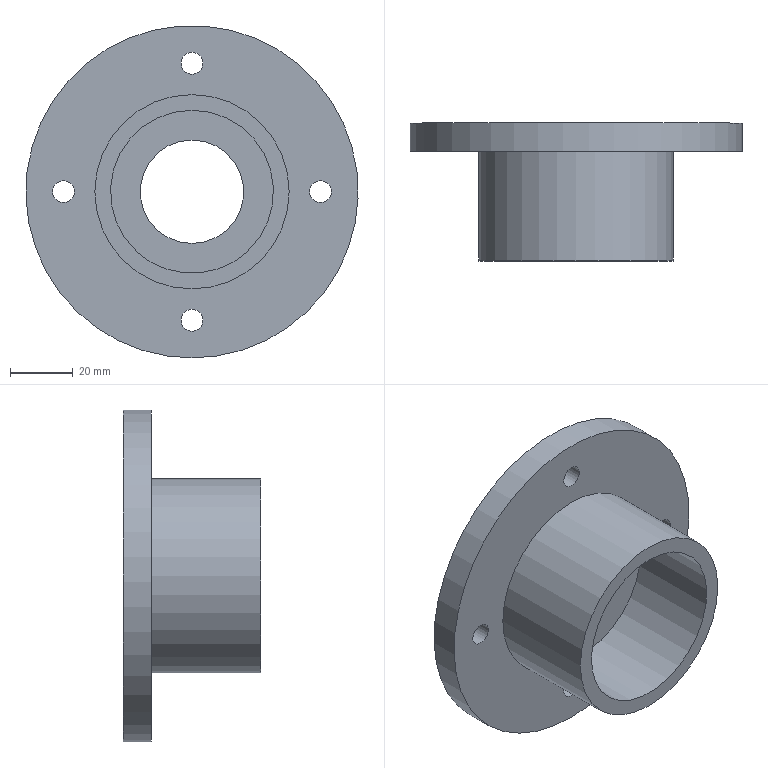Part | NX | features DATUM_CSYS 8, HOLE PACKAGE 7, SIMPLE HOLE 7, SKETCH 7, EXTRACT_DATUM_AXIS 4, EXTRACT_FACE 4, Instance Feature 3, EXTRUDE 2, OFFSET_REGION 1, Pattern Feature 1, SWP104 1 | 1 solid | 18 faces | box 106 x 44 x 106 mm | volume 98017 mm3 | cylinder 11 | plane 5 | cone 2 | commonest cylinder face diameters 7 x4 33 x2 48 x1 52 x1 58 x1 62 x1
STEP:
#1=CARTESIAN_POINT('',(0.,-14.,16.5));
#2=VERTEX_POINT('',#1);
#3=CARTESIAN_POINT('',(0.,-14.,0.));
#4=DIRECTION('',(0.,1.,0.));
#5=DIRECTION('',(0.,0.,1.));
#6=AXIS2_PLACEMENT_3D('',#3,#4,#5);
#7=CIRCLE('',#6,16.5);
#8=EDGE_CURVE('',#2,#2,#7,.T.);
#9=ORIENTED_EDGE('',*,*,#8,.F.);
#10=EDGE_LOOP('',(#9));
#11=FACE_BOUND('',#10,.T.);
#12=CARTESIAN_POINT('',(0.,-9.169,16.5));
#13=VERTEX_POINT('',#12);
#14=CARTESIAN_POINT('',(0.,-9.169,0.));
#15=DIRECTION('',(0.,1.,0.));
#16=DIRECTION('',(0.,0.,1.));
#17=AXIS2_PLACEMENT_3D('',#14,#15,#16);
#18=CIRCLE('',#17,16.5);
#19=EDGE_CURVE('',#13,#13,#18,.F.);
#20=ORIENTED_EDGE('',*,*,#19,.F.);
#21=EDGE_LOOP('',(#20));
#22=FACE_BOUND('',#21,.T.);
#23=CARTESIAN_POINT('',(0.,-44.,0.));
#24=DIRECTION('',(0.,1.,0.));
#25=DIRECTION('',(0.,0.,1.));
#26=AXIS2_PLACEMENT_3D('',#23,#24,#25);
#27=CYLINDRICAL_SURFACE('',#26,16.5);
#28=ADVANCED_FACE('',(#11,#22),#27,.F.);
#29=CARTESIAN_POINT('',(0.,-3.,-16.5));
#30=VERTEX_POINT('',#29);
#31=CARTESIAN_POINT('',(0.,-3.,0.));
#32=DIRECTION('',(0.,-1.,0.));
#33=DIRECTION('',(0.,0.,-1.));
#34=AXIS2_PLACEMENT_3D('',#31,#32,#33);
#35=CIRCLE('',#34,16.5);
#36=EDGE_CURVE('',#30,#30,#35,.F.);
#37=ORIENTED_EDGE('',*,*,#36,.T.);
#38=EDGE_LOOP('',(#37));
#39=FACE_BOUND('',#38,.T.);
#40=CARTESIAN_POINT('',(0.,-3.327,-16.5));
#41=VERTEX_POINT('',#40);
#42=CARTESIAN_POINT('',(0.,-3.327,0.));
#43=DIRECTION('',(0.,-1.,0.));
#44=DIRECTION('',(0.,0.,-1.));
#45=AXIS2_PLACEMENT_3D('',#42,#43,#44);
#46=CIRCLE('',#45,16.5);
#47=EDGE_CURVE('',#41,#41,#46,.F.);
#48=ORIENTED_EDGE('',*,*,#47,.F.);
#49=EDGE_LOOP('',(#48));
#50=FACE_BOUND('',#49,.T.);
#51=CARTESIAN_POINT('',(0.,-44.,0.));
#52=DIRECTION('',(0.,1.,0.));
#53=DIRECTION('',(0.,0.,1.));
#54=AXIS2_PLACEMENT_3D('',#51,#52,#53);
#55=CYLINDRICAL_SURFACE('',#54,16.5);
#56=ADVANCED_FACE('',(#39,#50),#55,.F.);
#57=CARTESIAN_POINT('',(0.,-9.,-53.));
#58=VERTEX_POINT('',#57);
#59=CARTESIAN_POINT('',(0.,-9.,0.));
#60=DIRECTION('',(0.,-1.,0.));
#61=DIRECTION('',(0.,0.,-1.));
#62=AXIS2_PLACEMENT_3D('',#59,#60,#61);
#63=CIRCLE('',#62,53.);
#64=EDGE_CURVE('',#58,#58,#63,.T.);
#65=ORIENTED_EDGE('',*,*,#64,.F.);
#66=EDGE_LOOP('',(#65));
#67=FACE_BOUND('',#66,.T.);
#68=CARTESIAN_POINT('',(0.,0.,-53.));
#69=VERTEX_POINT('',#68);
#70=CARTESIAN_POINT('',(0.,0.,0.));
#71=DIRECTION('',(0.,-1.,0.));
#72=DIRECTION('',(0.,0.,-1.));
#73=AXIS2_PLACEMENT_3D('',#70,#71,#72);
#74=CIRCLE('',#73,53.);
#75=EDGE_CURVE('',#69,#69,#74,.T.);
#76=ORIENTED_EDGE('',*,*,#75,.T.);
#77=EDGE_LOOP('',(#76));
#78=FACE_BOUND('',#77,.T.);
#79=CARTESIAN_POINT('',(0.,-9.,0.));
#80=DIRECTION('',(0.,1.,0.));
#81=DIRECTION('',(0.,0.,1.));
#82=AXIS2_PLACEMENT_3D('',#79,#80,#81);
#83=CYLINDRICAL_SURFACE('',#82,53.);
#84=ADVANCED_FACE('',(#67,#78),#83,.T.);
#85=CARTESIAN_POINT('',(0.,-9.,-44.5));
#86=VERTEX_POINT('',#85);
#87=CARTESIAN_POINT('',(0.,-9.,-41.));
#88=DIRECTION('',(0.,-1.,0.));
#89=DIRECTION('',(0.,0.,-1.));
#90=AXIS2_PLACEMENT_3D('',#87,#88,#89);
#91=CIRCLE('',#90,3.5);
#92=EDGE_CURVE('',#86,#86,#91,.T.);
#93=ORIENTED_EDGE('',*,*,#92,.F.);
#94=EDGE_LOOP('',(#93));
#95=FACE_BOUND('',#94,.T.);
#96=CARTESIAN_POINT('',(41.,-9.,-3.5));
#97=VERTEX_POINT('',#96);
#98=CARTESIAN_POINT('',(41.,-9.,0.));
#99=DIRECTION('',(0.,-1.,0.));
#100=DIRECTION('',(0.,0.,-1.));
#101=AXIS2_PLACEMENT_3D('',#98,#99,#100);
#102=CIRCLE('',#101,3.5);
#103=EDGE_CURVE('',#97,#97,#102,.T.);
#104=ORIENTED_EDGE('',*,*,#103,.F.);
#105=EDGE_LOOP('',(#104));
#106=FACE_BOUND('',#105,.T.);
#107=CARTESIAN_POINT('',(0.,-9.,37.5));
#108=VERTEX_POINT('',#107);
#109=CARTESIAN_POINT('',(0.,-9.,41.));
#110=DIRECTION('',(0.,-1.,0.));
#111=DIRECTION('',(0.,0.,-1.));
#112=AXIS2_PLACEMENT_3D('',#109,#110,#111);
#113=CIRCLE('',#112,3.5);
#114=EDGE_CURVE('',#108,#108,#113,.T.);
#115=ORIENTED_EDGE('',*,*,#114,.F.);
#116=EDGE_LOOP('',(#115));
#117=FACE_BOUND('',#116,.T.);
#118=CARTESIAN_POINT('',(-41.,-9.,-3.5));
#119=VERTEX_POINT('',#118);
#120=CARTESIAN_POINT('',(-41.,-9.,0.));
#121=DIRECTION('',(0.,-1.,0.));
#122=DIRECTION('',(0.,0.,-1.));
#123=AXIS2_PLACEMENT_3D('',#120,#121,#122);
#124=CIRCLE('',#123,3.5);
#125=EDGE_CURVE('',#119,#119,#124,.T.);
#126=ORIENTED_EDGE('',*,*,#125,.F.);
#127=EDGE_LOOP('',(#126));
#128=FACE_BOUND('',#127,.T.);
#129=CARTESIAN_POINT('',(31.,-9.,0.));
#130=VERTEX_POINT('',#129);
#131=CARTESIAN_POINT('',(0.,-9.,0.));
#132=DIRECTION('',(0.,-1.,0.));
#133=DIRECTION('',(1.,0.,0.));
#134=AXIS2_PLACEMENT_3D('',#131,#132,#133);
#135=CIRCLE('',#134,31.);
#136=EDGE_CURVE('',#130,#130,#135,.T.);
#137=ORIENTED_EDGE('',*,*,#136,.F.);
#138=EDGE_LOOP('',(#137));
#139=FACE_BOUND('',#138,.T.);
#140=ORIENTED_EDGE('',*,*,#64,.T.);
#141=EDGE_LOOP('',(#140));
#142=FACE_BOUND('',#141,.T.);
#143=CARTESIAN_POINT('',(0.,-9.,0.));
#144=DIRECTION('',(0.,-1.,0.));
#145=DIRECTION('',(0.,0.,-1.));
#146=AXIS2_PLACEMENT_3D('',#143,#144,#145);
#147=PLANE('',#146);
#148=ADVANCED_FACE('',(#95,#106,#117,#128,#139,#142),#147,.T.);
#149=CARTESIAN_POINT('',(0.,0.,-44.5));
#150=VERTEX_POINT('',#149);
#151=CARTESIAN_POINT('',(0.,0.,-41.));
#152=DIRECTION('',(0.,-1.,0.));
#153=DIRECTION('',(0.,0.,-1.));
#154=AXIS2_PLACEMENT_3D('',#151,#152,#153);
#155=CIRCLE('',#154,3.5);
#156=EDGE_CURVE('',#150,#150,#155,.T.);
#157=ORIENTED_EDGE('',*,*,#156,.T.);
#158=EDGE_LOOP('',(#157));
#159=FACE_BOUND('',#158,.T.);
#160=CARTESIAN_POINT('',(41.,0.,-3.5));
#161=VERTEX_POINT('',#160);
#162=CARTESIAN_POINT('',(41.,0.,0.));
#163=DIRECTION('',(0.,-1.,0.));
#164=DIRECTION('',(0.,0.,-1.));
#165=AXIS2_PLACEMENT_3D('',#162,#163,#164);
#166=CIRCLE('',#165,3.5);
#167=EDGE_CURVE('',#161,#161,#166,.T.);
#168=ORIENTED_EDGE('',*,*,#167,.T.);
#169=EDGE_LOOP('',(#168));
#170=FACE_BOUND('',#169,.T.);
#171=CARTESIAN_POINT('',(0.,0.,37.5));
#172=VERTEX_POINT('',#171);
#173=CARTESIAN_POINT('',(0.,0.,41.));
#174=DIRECTION('',(0.,-1.,0.));
#175=DIRECTION('',(0.,0.,-1.));
#176=AXIS2_PLACEMENT_3D('',#173,#174,#175);
#177=CIRCLE('',#176,3.5);
#178=EDGE_CURVE('',#172,#172,#177,.T.);
#179=ORIENTED_EDGE('',*,*,#178,.T.);
#180=EDGE_LOOP('',(#179));
#181=FACE_BOUND('',#180,.T.);
#182=CARTESIAN_POINT('',(-41.,0.,-3.5));
#183=VERTEX_POINT('',#182);
#184=CARTESIAN_POINT('',(-41.,0.,0.));
#185=DIRECTION('',(0.,-1.,0.));
#186=DIRECTION('',(0.,0.,-1.));
#187=AXIS2_PLACEMENT_3D('',#184,#185,#186);
#188=CIRCLE('',#187,3.5);
#189=EDGE_CURVE('',#183,#183,#188,.T.);
#190=ORIENTED_EDGE('',*,*,#189,.T.);
#191=EDGE_LOOP('',(#190));
#192=FACE_BOUND('',#191,.T.);
#193=CARTESIAN_POINT('',(0.,0.,-29.));
#194=VERTEX_POINT('',#193);
#195=CARTESIAN_POINT('',(0.,0.,0.));
#196=DIRECTION('',(0.,-1.,0.));
#197=DIRECTION('',(0.,0.,-1.));
#198=AXIS2_PLACEMENT_3D('',#195,#196,#197);
#199=CIRCLE('',#198,29.);
#200=EDGE_CURVE('',#194,#194,#199,.T.);
#201=ORIENTED_EDGE('',*,*,#200,.T.);
#202=EDGE_LOOP('',(#201));
#203=FACE_BOUND('',#202,.T.);
#204=ORIENTED_EDGE('',*,*,#75,.F.);
#205=EDGE_LOOP('',(#204));
#206=FACE_BOUND('',#205,.T.);
#207=CARTESIAN_POINT('',(0.,0.,0.));
#208=DIRECTION('',(0.,-1.,0.));
#209=DIRECTION('',(0.,0.,-1.));
#210=AXIS2_PLACEMENT_3D('',#207,#208,#209);
#211=PLANE('',#210);
#212=ADVANCED_FACE('',(#159,#170,#181,#192,#203,#206),#211,.F.);
#213=CARTESIAN_POINT('',(31.,-44.,0.));
#214=VERTEX_POINT('',#213);
#215=CARTESIAN_POINT('',(0.,-44.,0.));
#216=DIRECTION('',(0.,-1.,0.));
#217=DIRECTION('',(1.,0.,0.));
#218=AXIS2_PLACEMENT_3D('',#215,#216,#217);
#219=CIRCLE('',#218,31.);
#220=EDGE_CURVE('',#214,#214,#219,.T.);
#221=ORIENTED_EDGE('',*,*,#220,.F.);
#222=EDGE_LOOP('',(#221));
#223=FACE_BOUND('',#222,.T.);
#224=ORIENTED_EDGE('',*,*,#136,.T.);
#225=EDGE_LOOP('',(#224));
#226=FACE_BOUND('',#225,.T.);
#227=CARTESIAN_POINT('',(0.,-44.,0.));
#228=DIRECTION('',(0.,1.,0.));
#229=DIRECTION('',(0.,0.,1.));
#230=AXIS2_PLACEMENT_3D('',#227,#228,#229);
#231=CYLINDRICAL_SURFACE('',#230,31.);
#232=ADVANCED_FACE('',(#223,#226),#231,.T.);
#233=CARTESIAN_POINT('',(0.,-44.,26.));
#234=VERTEX_POINT('',#233);
#235=CARTESIAN_POINT('',(0.,-44.,0.));
#236=DIRECTION('',(0.,1.,0.));
#237=DIRECTION('',(0.,0.,1.));
#238=AXIS2_PLACEMENT_3D('',#235,#236,#237);
#239=CIRCLE('',#238,26.);
#240=EDGE_CURVE('',#234,#234,#239,.T.);
#241=ORIENTED_EDGE('',*,*,#240,.T.);
#242=EDGE_LOOP('',(#241));
#243=FACE_BOUND('',#242,.T.);
#244=ORIENTED_EDGE('',*,*,#220,.T.);
#245=EDGE_LOOP('',(#244));
#246=FACE_BOUND('',#245,.T.);
#247=CARTESIAN_POINT('',(0.,-44.,0.));
#248=DIRECTION('',(0.,-1.,0.));
#249=DIRECTION('',(0.,0.,-1.));
#250=AXIS2_PLACEMENT_3D('',#247,#248,#249);
#251=PLANE('',#250);
#252=ADVANCED_FACE('',(#243,#246),#251,.T.);
#253=ORIENTED_EDGE('',*,*,#8,.T.);
#254=EDGE_LOOP('',(#253));
#255=FACE_BOUND('',#254,.T.);
#256=CARTESIAN_POINT('',(0.,-14.,26.));
#257=VERTEX_POINT('',#256);
#258=CARTESIAN_POINT('',(0.,-14.,0.));
#259=DIRECTION('',(0.,1.,0.));
#260=DIRECTION('',(0.,0.,1.));
#261=AXIS2_PLACEMENT_3D('',#258,#259,#260);
#262=CIRCLE('',#261,26.);
#263=EDGE_CURVE('',#257,#257,#262,.F.);
#264=ORIENTED_EDGE('',*,*,#263,.T.);
#265=EDGE_LOOP('',(#264));
#266=FACE_BOUND('',#265,.T.);
#267=CARTESIAN_POINT('',(0.,-14.,0.));
#268=DIRECTION('',(0.,1.,0.));
#269=DIRECTION('',(0.,0.,1.));
#270=AXIS2_PLACEMENT_3D('',#267,#268,#269);
#271=PLANE('',#270);
#272=ADVANCED_FACE('',(#255,#266),#271,.F.);
#273=ORIENTED_EDGE('',*,*,#263,.F.);
#274=EDGE_LOOP('',(#273));
#275=FACE_BOUND('',#274,.T.);
#276=ORIENTED_EDGE('',*,*,#240,.F.);
#277=EDGE_LOOP('',(#276));
#278=FACE_BOUND('',#277,.T.);
#279=CARTESIAN_POINT('',(0.,-44.,0.));
#280=DIRECTION('',(0.,1.,0.));
#281=DIRECTION('',(0.,0.,1.));
#282=AXIS2_PLACEMENT_3D('',#279,#280,#281);
#283=CYLINDRICAL_SURFACE('',#282,26.);
#284=ADVANCED_FACE('',(#275,#278),#283,.F.);
#285=CARTESIAN_POINT('',(0.,-3.,-29.));
#286=VERTEX_POINT('',#285);
#287=CARTESIAN_POINT('',(0.,-3.,0.));
#288=DIRECTION('',(0.,-1.,0.));
#289=DIRECTION('',(0.,0.,-1.));
#290=AXIS2_PLACEMENT_3D('',#287,#288,#289);
#291=CIRCLE('',#290,29.);
#292=EDGE_CURVE('',#286,#286,#291,.F.);
#293=ORIENTED_EDGE('',*,*,#292,.T.);
#294=EDGE_LOOP('',(#293));
#295=FACE_BOUND('',#294,.T.);
#296=ORIENTED_EDGE('',*,*,#36,.F.);
#297=EDGE_LOOP('',(#296));
#298=FACE_BOUND('',#297,.T.);
#299=CARTESIAN_POINT('',(0.,-3.,0.));
#300=DIRECTION('',(0.,-1.,0.));
#301=DIRECTION('',(0.,0.,-1.));
#302=AXIS2_PLACEMENT_3D('',#299,#300,#301);
#303=PLANE('',#302);
#304=ADVANCED_FACE('',(#295,#298),#303,.F.);
#305=ORIENTED_EDGE('',*,*,#292,.F.);
#306=EDGE_LOOP('',(#305));
#307=FACE_BOUND('',#306,.T.);
#308=ORIENTED_EDGE('',*,*,#200,.F.);
#309=EDGE_LOOP('',(#308));
#310=FACE_BOUND('',#309,.T.);
#311=CARTESIAN_POINT('',(0.,0.,0.));
#312=DIRECTION('',(0.,-1.,0.));
#313=DIRECTION('',(0.,0.,-1.));
#314=AXIS2_PLACEMENT_3D('',#311,#312,#313);
#315=CYLINDRICAL_SURFACE('',#314,29.);
#316=ADVANCED_FACE('',(#307,#310),#315,.F.);
#317=CARTESIAN_POINT('',(0.,-8.248,-24.));
#318=VERTEX_POINT('',#317);
#319=CARTESIAN_POINT('',(0.,-8.248,0.));
#320=DIRECTION('',(0.,-1.,0.));
#321=DIRECTION('',(0.,0.,-1.));
#322=AXIS2_PLACEMENT_3D('',#319,#320,#321);
#323=CIRCLE('',#322,24.);
#324=EDGE_CURVE('',#318,#318,#323,.F.);
#325=ORIENTED_EDGE('',*,*,#324,.T.);
#326=EDGE_LOOP('',(#325));
#327=FACE_BOUND('',#326,.T.);
#328=ORIENTED_EDGE('',*,*,#19,.T.);
#329=EDGE_LOOP('',(#328));
#330=FACE_BOUND('',#329,.T.);
#331=CARTESIAN_POINT('',(0.,-8.248,0.));
#332=DIRECTION('',(0.,1.,0.));
#333=DIRECTION('',(0.,0.,1.));
#334=AXIS2_PLACEMENT_3D('',#331,#332,#333);
#335=CONICAL_SURFACE('',#334,24.,1.449);
#336=ADVANCED_FACE('',(#327,#330),#335,.F.);
#337=CARTESIAN_POINT('',(0.,-4.248,-24.));
#338=VERTEX_POINT('',#337);
#339=CARTESIAN_POINT('',(0.,-4.248,0.));
#340=DIRECTION('',(0.,-1.,0.));
#341=DIRECTION('',(0.,0.,-1.));
#342=AXIS2_PLACEMENT_3D('',#339,#340,#341);
#343=CIRCLE('',#342,24.);
#344=EDGE_CURVE('',#338,#338,#343,.F.);
#345=ORIENTED_EDGE('',*,*,#344,.F.);
#346=EDGE_LOOP('',(#345));
#347=FACE_BOUND('',#346,.T.);
#348=ORIENTED_EDGE('',*,*,#47,.T.);
#349=EDGE_LOOP('',(#348));
#350=FACE_BOUND('',#349,.T.);
#351=CARTESIAN_POINT('',(0.,-3.266,0.));
#352=DIRECTION('',(0.,-1.,0.));
#353=DIRECTION('',(0.,0.,-1.));
#354=AXIS2_PLACEMENT_3D('',#351,#352,#353);
#355=CONICAL_SURFACE('',#354,16.,1.449);
#356=ADVANCED_FACE('',(#347,#350),#355,.F.);
#357=ORIENTED_EDGE('',*,*,#324,.F.);
#358=EDGE_LOOP('',(#357));
#359=FACE_BOUND('',#358,.T.);
#360=ORIENTED_EDGE('',*,*,#344,.T.);
#361=EDGE_LOOP('',(#360));
#362=FACE_BOUND('',#361,.T.);
#363=CARTESIAN_POINT('',(0.,0.,0.));
#364=DIRECTION('',(0.,-1.,0.));
#365=DIRECTION('',(0.,0.,-1.));
#366=AXIS2_PLACEMENT_3D('',#363,#364,#365);
#367=CYLINDRICAL_SURFACE('',#366,24.);
#368=ADVANCED_FACE('',(#359,#362),#367,.F.);
#369=ORIENTED_EDGE('',*,*,#125,.T.);
#370=EDGE_LOOP('',(#369));
#371=FACE_BOUND('',#370,.T.);
#372=ORIENTED_EDGE('',*,*,#189,.F.);
#373=EDGE_LOOP('',(#372));
#374=FACE_BOUND('',#373,.T.);
#375=CARTESIAN_POINT('',(-41.,0.,0.));
#376=DIRECTION('',(0.,-1.,0.));
#377=DIRECTION('',(0.,0.,-1.));
#378=AXIS2_PLACEMENT_3D('',#375,#376,#377);
#379=CYLINDRICAL_SURFACE('',#378,3.5);
#380=ADVANCED_FACE('',(#371,#374),#379,.F.);
#381=ORIENTED_EDGE('',*,*,#114,.T.);
#382=EDGE_LOOP('',(#381));
#383=FACE_BOUND('',#382,.T.);
#384=ORIENTED_EDGE('',*,*,#178,.F.);
#385=EDGE_LOOP('',(#384));
#386=FACE_BOUND('',#385,.T.);
#387=CARTESIAN_POINT('',(0.,0.,41.));
#388=DIRECTION('',(0.,-1.,0.));
#389=DIRECTION('',(0.,0.,-1.));
#390=AXIS2_PLACEMENT_3D('',#387,#388,#389);
#391=CYLINDRICAL_SURFACE('',#390,3.5);
#392=ADVANCED_FACE('',(#383,#386),#391,.F.);
#393=ORIENTED_EDGE('',*,*,#103,.T.);
#394=EDGE_LOOP('',(#393));
#395=FACE_BOUND('',#394,.T.);
#396=ORIENTED_EDGE('',*,*,#167,.F.);
#397=EDGE_LOOP('',(#396));
#398=FACE_BOUND('',#397,.T.);
#399=CARTESIAN_POINT('',(41.,0.,0.));
#400=DIRECTION('',(0.,-1.,0.));
#401=DIRECTION('',(0.,0.,-1.));
#402=AXIS2_PLACEMENT_3D('',#399,#400,#401);
#403=CYLINDRICAL_SURFACE('',#402,3.5);
#404=ADVANCED_FACE('',(#395,#398),#403,.F.);
#405=ORIENTED_EDGE('',*,*,#92,.T.);
#406=EDGE_LOOP('',(#405));
#407=FACE_BOUND('',#406,.T.);
#408=ORIENTED_EDGE('',*,*,#156,.F.);
#409=EDGE_LOOP('',(#408));
#410=FACE_BOUND('',#409,.T.);
#411=CARTESIAN_POINT('',(0.,0.,-41.));
#412=DIRECTION('',(0.,-1.,0.));
#413=DIRECTION('',(0.,0.,-1.));
#414=AXIS2_PLACEMENT_3D('',#411,#412,#413);
#415=CYLINDRICAL_SURFACE('',#414,3.5);
#416=ADVANCED_FACE('',(#407,#410),#415,.F.);
#417=CLOSED_SHELL('',(#28,#56,#84,#148,#212,#232,#252,#272,#284,#304,#316,#336,#356,#368,#380,#392,#404,#416));
#418=MANIFOLD_SOLID_BREP('',#417);
#419=(LENGTH_UNIT()NAMED_UNIT(*)SI_UNIT(.MILLI.,.METRE.));
#420=UNCERTAINTY_MEASURE_WITH_UNIT(LENGTH_MEASURE(0.00001),#419,'','');
#421=(NAMED_UNIT(*)PLANE_ANGLE_UNIT()SI_UNIT($,.RADIAN.));
#422=(NAMED_UNIT(*)SI_UNIT($,.STERADIAN.)SOLID_ANGLE_UNIT());
#423=(GEOMETRIC_REPRESENTATION_CONTEXT(3)GLOBAL_UNCERTAINTY_ASSIGNED_CONTEXT((#420))GLOBAL_UNIT_ASSIGNED_CONTEXT((#419,#421,#422))REPRESENTATION_CONTEXT('',''));
#424=ADVANCED_BREP_SHAPE_REPRESENTATION('',(#418),#423);